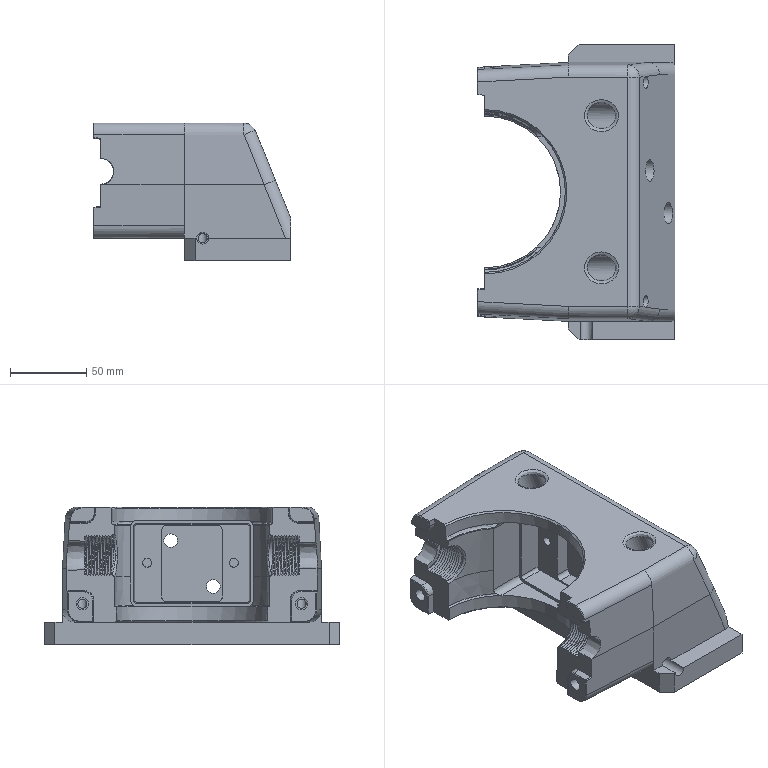Part | NX | features solid 2 | 1 solid | 284 faces | box 130 x 194 x 90.5 mm | volume 1109327 mm3 | plane 114 | cylinder 80 | spline 61 | cone 17 | torus 6 | sphere 6 | commonest cylinder face diameters 6 x31 8 x13 16 x11 4 x4 8.04 x4 12 x4